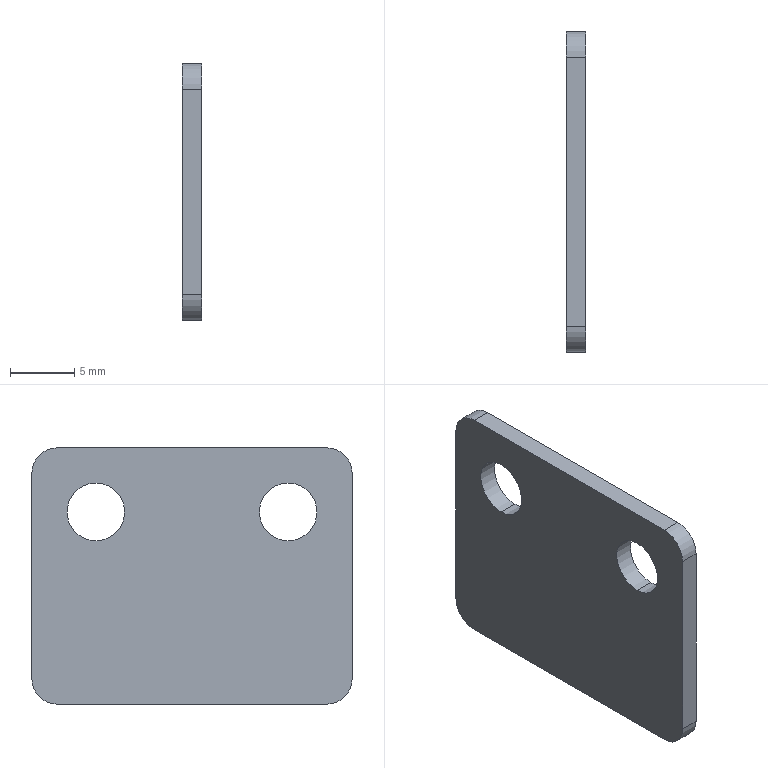Part | SolidWorks | features BaseBody 1 | 1 solid | 14 faces | box 1.5 x 25 x 20 mm | volume 697.137 mm3 | cylinder 8 | plane 6 | commonest cylinder face diameters 4 x4 4.5 x4
STEP:
#1=CARTESIAN_POINT('',(0.,12.5,-2.));
#2=VERTEX_POINT('',#1);
#3=CARTESIAN_POINT('',(0.,10.5,0.));
#4=VERTEX_POINT('',#3);
#5=CARTESIAN_POINT('',(0.,10.5,-2.));
#6=DIRECTION('',(1.,0.,0.));
#7=DIRECTION('',(0.,0.,-1.));
#8=AXIS2_PLACEMENT_3D('',#5,#6,#7);
#9=CIRCLE('',#8,2.);
#10=EDGE_CURVE('',#2,#4,#9,.T.);
#11=ORIENTED_EDGE('',*,*,#10,.F.);
#12=CARTESIAN_POINT('',(-1.5,12.5,-2.));
#13=VERTEX_POINT('',#12);
#14=CARTESIAN_POINT('',(0.,12.5,-2.));
#15=DIRECTION('',(1.,0.,0.));
#16=VECTOR('',#15,1000.);
#17=LINE('',#14,#16);
#18=EDGE_CURVE('',#13,#2,#17,.T.);
#19=ORIENTED_EDGE('',*,*,#18,.F.);
#20=CARTESIAN_POINT('',(-1.5,10.5,0.));
#21=VERTEX_POINT('',#20);
#22=CARTESIAN_POINT('',(-1.5,10.5,-2.));
#23=DIRECTION('',(-1.,0.,0.));
#24=DIRECTION('',(0.,0.,-1.));
#25=AXIS2_PLACEMENT_3D('',#22,#23,#24);
#26=CIRCLE('',#25,2.);
#27=EDGE_CURVE('',#21,#13,#26,.T.);
#28=ORIENTED_EDGE('',*,*,#27,.F.);
#29=CARTESIAN_POINT('',(0.,10.5,0.));
#30=DIRECTION('',(-1.,0.,0.));
#31=VECTOR('',#30,1000.);
#32=LINE('',#29,#31);
#33=EDGE_CURVE('',#4,#21,#32,.T.);
#34=ORIENTED_EDGE('',*,*,#33,.F.);
#35=EDGE_LOOP('',(#11,#19,#28,#34));
#36=FACE_OUTER_BOUND('',#35,.T.);
#37=CARTESIAN_POINT('',(0.,10.5,-2.));
#38=DIRECTION('',(-1.,0.,0.));
#39=DIRECTION('',(0.,0.,1.));
#40=AXIS2_PLACEMENT_3D('',#37,#38,#39);
#41=CYLINDRICAL_SURFACE('',#40,2.);
#42=ADVANCED_FACE('',(#36),#41,.T.);
#43=CARTESIAN_POINT('',(0.,-10.5,0.));
#44=VERTEX_POINT('',#43);
#45=CARTESIAN_POINT('',(0.,-12.5,-2.));
#46=VERTEX_POINT('',#45);
#47=CARTESIAN_POINT('',(0.,-10.5,-2.));
#48=DIRECTION('',(1.,0.,0.));
#49=DIRECTION('',(0.,0.,-1.));
#50=AXIS2_PLACEMENT_3D('',#47,#48,#49);
#51=CIRCLE('',#50,2.);
#52=EDGE_CURVE('',#44,#46,#51,.T.);
#53=ORIENTED_EDGE('',*,*,#52,.F.);
#54=CARTESIAN_POINT('',(-1.5,-10.5,0.));
#55=VERTEX_POINT('',#54);
#56=CARTESIAN_POINT('',(0.,-10.5,0.));
#57=DIRECTION('',(1.,0.,0.));
#58=VECTOR('',#57,1000.);
#59=LINE('',#56,#58);
#60=EDGE_CURVE('',#55,#44,#59,.T.);
#61=ORIENTED_EDGE('',*,*,#60,.F.);
#62=CARTESIAN_POINT('',(-1.5,-12.5,-2.));
#63=VERTEX_POINT('',#62);
#64=CARTESIAN_POINT('',(-1.5,-10.5,-2.));
#65=DIRECTION('',(-1.,0.,0.));
#66=DIRECTION('',(0.,0.,-1.));
#67=AXIS2_PLACEMENT_3D('',#64,#65,#66);
#68=CIRCLE('',#67,2.);
#69=EDGE_CURVE('',#63,#55,#68,.T.);
#70=ORIENTED_EDGE('',*,*,#69,.F.);
#71=CARTESIAN_POINT('',(-1.5,-12.5,-2.));
#72=DIRECTION('',(-1.,0.,0.));
#73=VECTOR('',#72,1000.);
#74=LINE('',#71,#73);
#75=EDGE_CURVE('',#46,#63,#74,.T.);
#76=ORIENTED_EDGE('',*,*,#75,.F.);
#77=EDGE_LOOP('',(#53,#61,#70,#76));
#78=FACE_OUTER_BOUND('',#77,.T.);
#79=CARTESIAN_POINT('',(0.,-10.5,-2.));
#80=DIRECTION('',(1.,0.,0.));
#81=DIRECTION('',(0.,0.,-1.));
#82=AXIS2_PLACEMENT_3D('',#79,#80,#81);
#83=CYLINDRICAL_SURFACE('',#82,2.);
#84=ADVANCED_FACE('',(#78),#83,.T.);
#85=CARTESIAN_POINT('',(-1.5,12.5,-18.));
#86=VERTEX_POINT('',#85);
#87=CARTESIAN_POINT('',(-1.5,10.5,-20.));
#88=VERTEX_POINT('',#87);
#89=CARTESIAN_POINT('',(-1.5,10.5,-18.));
#90=DIRECTION('',(-1.,0.,0.));
#91=DIRECTION('',(0.,0.,-1.));
#92=AXIS2_PLACEMENT_3D('',#89,#90,#91);
#93=CIRCLE('',#92,2.);
#94=EDGE_CURVE('',#86,#88,#93,.T.);
#95=ORIENTED_EDGE('',*,*,#94,.F.);
#96=CARTESIAN_POINT('',(0.,12.5,-18.));
#97=VERTEX_POINT('',#96);
#98=CARTESIAN_POINT('',(0.,12.5,-18.));
#99=DIRECTION('',(-1.,0.,0.));
#100=VECTOR('',#99,1000.);
#101=LINE('',#98,#100);
#102=EDGE_CURVE('',#97,#86,#101,.T.);
#103=ORIENTED_EDGE('',*,*,#102,.F.);
#104=CARTESIAN_POINT('',(0.,10.5,-20.));
#105=VERTEX_POINT('',#104);
#106=CARTESIAN_POINT('',(0.,10.5,-18.));
#107=DIRECTION('',(1.,0.,0.));
#108=DIRECTION('',(0.,0.,-1.));
#109=AXIS2_PLACEMENT_3D('',#106,#107,#108);
#110=CIRCLE('',#109,2.);
#111=EDGE_CURVE('',#105,#97,#110,.T.);
#112=ORIENTED_EDGE('',*,*,#111,.F.);
#113=CARTESIAN_POINT('',(-1.5,10.5,-20.));
#114=DIRECTION('',(1.,0.,0.));
#115=VECTOR('',#114,1000.);
#116=LINE('',#113,#115);
#117=EDGE_CURVE('',#88,#105,#116,.T.);
#118=ORIENTED_EDGE('',*,*,#117,.F.);
#119=EDGE_LOOP('',(#95,#103,#112,#118));
#120=FACE_OUTER_BOUND('',#119,.T.);
#121=CARTESIAN_POINT('',(-1.5,10.5,-18.));
#122=DIRECTION('',(1.,0.,0.));
#123=DIRECTION('',(0.,0.,-1.));
#124=AXIS2_PLACEMENT_3D('',#121,#122,#123);
#125=CYLINDRICAL_SURFACE('',#124,2.);
#126=ADVANCED_FACE('',(#120),#125,.T.);
#127=CARTESIAN_POINT('',(-1.5,-10.5,-20.));
#128=VERTEX_POINT('',#127);
#129=CARTESIAN_POINT('',(-1.5,-12.5,-18.));
#130=VERTEX_POINT('',#129);
#131=CARTESIAN_POINT('',(-1.5,-10.5,-18.));
#132=DIRECTION('',(-1.,0.,0.));
#133=DIRECTION('',(0.,0.,-1.));
#134=AXIS2_PLACEMENT_3D('',#131,#132,#133);
#135=CIRCLE('',#134,2.);
#136=EDGE_CURVE('',#128,#130,#135,.T.);
#137=ORIENTED_EDGE('',*,*,#136,.F.);
#138=CARTESIAN_POINT('',(0.,-10.5,-20.));
#139=VERTEX_POINT('',#138);
#140=CARTESIAN_POINT('',(-1.5,-10.5,-20.));
#141=DIRECTION('',(-1.,0.,0.));
#142=VECTOR('',#141,1000.);
#143=LINE('',#140,#142);
#144=EDGE_CURVE('',#139,#128,#143,.T.);
#145=ORIENTED_EDGE('',*,*,#144,.F.);
#146=CARTESIAN_POINT('',(0.,-12.5,-18.));
#147=VERTEX_POINT('',#146);
#148=CARTESIAN_POINT('',(0.,-10.5,-18.));
#149=DIRECTION('',(1.,0.,0.));
#150=DIRECTION('',(0.,0.,-1.));
#151=AXIS2_PLACEMENT_3D('',#148,#149,#150);
#152=CIRCLE('',#151,2.);
#153=EDGE_CURVE('',#147,#139,#152,.T.);
#154=ORIENTED_EDGE('',*,*,#153,.F.);
#155=CARTESIAN_POINT('',(0.,-12.5,-18.));
#156=DIRECTION('',(1.,0.,0.));
#157=VECTOR('',#156,1000.);
#158=LINE('',#155,#157);
#159=EDGE_CURVE('',#130,#147,#158,.T.);
#160=ORIENTED_EDGE('',*,*,#159,.F.);
#161=EDGE_LOOP('',(#137,#145,#154,#160));
#162=FACE_OUTER_BOUND('',#161,.T.);
#163=CARTESIAN_POINT('',(0.,-10.5,-18.));
#164=DIRECTION('',(-1.,0.,0.));
#165=DIRECTION('',(0.,0.,1.));
#166=AXIS2_PLACEMENT_3D('',#163,#164,#165);
#167=CYLINDRICAL_SURFACE('',#166,2.);
#168=ADVANCED_FACE('',(#162),#167,.T.);
#169=CARTESIAN_POINT('',(-1.5,-7.5,-2.75));
#170=VERTEX_POINT('',#169);
#171=CARTESIAN_POINT('',(0.,-7.5,-2.75));
#172=VERTEX_POINT('',#171);
#173=CARTESIAN_POINT('',(0.,-7.5,-2.75));
#174=DIRECTION('',(1.,0.,0.));
#175=VECTOR('',#174,1000.);
#176=LINE('',#173,#175);
#177=EDGE_CURVE('',#170,#172,#176,.T.);
#178=ORIENTED_EDGE('',*,*,#177,.F.);
#179=CARTESIAN_POINT('',(-1.5,-7.5,-7.25));
#180=VERTEX_POINT('',#179);
#181=CARTESIAN_POINT('',(-1.5,-7.5,-5.));
#182=DIRECTION('',(1.,0.,0.));
#183=DIRECTION('',(0.,0.,-1.));
#184=AXIS2_PLACEMENT_3D('',#181,#182,#183);
#185=CIRCLE('',#184,2.25);
#186=EDGE_CURVE('',#180,#170,#185,.T.);
#187=ORIENTED_EDGE('',*,*,#186,.F.);
#188=CARTESIAN_POINT('',(0.,-7.5,-7.25));
#189=VERTEX_POINT('',#188);
#190=CARTESIAN_POINT('',(0.,-7.5,-7.25));
#191=DIRECTION('',(1.,0.,0.));
#192=VECTOR('',#191,1000.);
#193=LINE('',#190,#192);
#194=EDGE_CURVE('',#180,#189,#193,.T.);
#195=ORIENTED_EDGE('',*,*,#194,.T.);
#196=CARTESIAN_POINT('',(0.,-7.5,-5.));
#197=DIRECTION('',(1.,0.,0.));
#198=DIRECTION('',(0.,0.,-1.));
#199=AXIS2_PLACEMENT_3D('',#196,#197,#198);
#200=CIRCLE('',#199,2.25);
#201=EDGE_CURVE('',#189,#172,#200,.T.);
#202=ORIENTED_EDGE('',*,*,#201,.T.);
#203=EDGE_LOOP('',(#178,#187,#195,#202));
#204=FACE_OUTER_BOUND('',#203,.T.);
#205=CARTESIAN_POINT('',(0.,-7.5,-5.));
#206=DIRECTION('',(1.,0.,0.));
#207=DIRECTION('',(0.,0.,-1.));
#208=AXIS2_PLACEMENT_3D('',#205,#206,#207);
#209=CYLINDRICAL_SURFACE('',#208,2.25);
#210=ADVANCED_FACE('',(#204),#209,.F.);
#211=CARTESIAN_POINT('',(-1.5,7.5,-2.75));
#212=VERTEX_POINT('',#211);
#213=CARTESIAN_POINT('',(0.,7.5,-2.75));
#214=VERTEX_POINT('',#213);
#215=CARTESIAN_POINT('',(0.,7.5,-2.75));
#216=DIRECTION('',(1.,0.,0.));
#217=VECTOR('',#216,1000.);
#218=LINE('',#215,#217);
#219=EDGE_CURVE('',#212,#214,#218,.T.);
#220=ORIENTED_EDGE('',*,*,#219,.F.);
#221=CARTESIAN_POINT('',(-1.5,7.5,-7.25));
#222=VERTEX_POINT('',#221);
#223=CARTESIAN_POINT('',(-1.5,7.5,-5.));
#224=DIRECTION('',(1.,0.,0.));
#225=DIRECTION('',(0.,0.,-1.));
#226=AXIS2_PLACEMENT_3D('',#223,#224,#225);
#227=CIRCLE('',#226,2.25);
#228=EDGE_CURVE('',#222,#212,#227,.T.);
#229=ORIENTED_EDGE('',*,*,#228,.F.);
#230=CARTESIAN_POINT('',(0.,7.5,-7.25));
#231=VERTEX_POINT('',#230);
#232=CARTESIAN_POINT('',(0.,7.5,-7.25));
#233=DIRECTION('',(1.,0.,0.));
#234=VECTOR('',#233,1000.);
#235=LINE('',#232,#234);
#236=EDGE_CURVE('',#222,#231,#235,.T.);
#237=ORIENTED_EDGE('',*,*,#236,.T.);
#238=CARTESIAN_POINT('',(0.,7.5,-5.));
#239=DIRECTION('',(1.,0.,0.));
#240=DIRECTION('',(0.,0.,-1.));
#241=AXIS2_PLACEMENT_3D('',#238,#239,#240);
#242=CIRCLE('',#241,2.25);
#243=EDGE_CURVE('',#231,#214,#242,.T.);
#244=ORIENTED_EDGE('',*,*,#243,.T.);
#245=EDGE_LOOP('',(#220,#229,#237,#244));
#246=FACE_OUTER_BOUND('',#245,.T.);
#247=CARTESIAN_POINT('',(0.,7.5,-5.));
#248=DIRECTION('',(1.,0.,0.));
#249=DIRECTION('',(0.,0.,-1.));
#250=AXIS2_PLACEMENT_3D('',#247,#248,#249);
#251=CYLINDRICAL_SURFACE('',#250,2.25);
#252=ADVANCED_FACE('',(#246),#251,.F.);
#253=CARTESIAN_POINT('',(-1.5,-12.5,-20.));
#254=DIRECTION('',(0.,0.,1.));
#255=VECTOR('',#254,1000.);
#256=LINE('',#253,#255);
#257=EDGE_CURVE('',#130,#63,#256,.T.);
#258=ORIENTED_EDGE('',*,*,#257,.F.);
#259=ORIENTED_EDGE('',*,*,#159,.T.);
#260=CARTESIAN_POINT('',(0.,-12.5,-20.));
#261=DIRECTION('',(0.,0.,1.));
#262=VECTOR('',#261,1000.);
#263=LINE('',#260,#262);
#264=EDGE_CURVE('',#147,#46,#263,.T.);
#265=ORIENTED_EDGE('',*,*,#264,.T.);
#266=ORIENTED_EDGE('',*,*,#75,.T.);
#267=EDGE_LOOP('',(#258,#259,#265,#266));
#268=FACE_OUTER_BOUND('',#267,.T.);
#269=CARTESIAN_POINT('',(0.,-12.5,0.));
#270=DIRECTION('',(0.,1.,0.));
#271=DIRECTION('',(1.,0.,0.));
#272=AXIS2_PLACEMENT_3D('',#269,#270,#271);
#273=PLANE('',#272);
#274=ADVANCED_FACE('',(#268),#273,.F.);
#275=CARTESIAN_POINT('',(0.,12.5,-20.));
#276=DIRECTION('',(0.,0.,1.));
#277=VECTOR('',#276,1000.);
#278=LINE('',#275,#277);
#279=EDGE_CURVE('',#97,#2,#278,.T.);
#280=ORIENTED_EDGE('',*,*,#279,.F.);
#281=ORIENTED_EDGE('',*,*,#102,.T.);
#282=CARTESIAN_POINT('',(-1.5,12.5,-20.));
#283=DIRECTION('',(0.,0.,1.));
#284=VECTOR('',#283,1000.);
#285=LINE('',#282,#284);
#286=EDGE_CURVE('',#86,#13,#285,.T.);
#287=ORIENTED_EDGE('',*,*,#286,.T.);
#288=ORIENTED_EDGE('',*,*,#18,.T.);
#289=EDGE_LOOP('',(#280,#281,#287,#288));
#290=FACE_OUTER_BOUND('',#289,.T.);
#291=CARTESIAN_POINT('',(0.,12.5,0.));
#292=DIRECTION('',(0.,1.,0.));
#293=DIRECTION('',(1.,0.,0.));
#294=AXIS2_PLACEMENT_3D('',#291,#292,#293);
#295=PLANE('',#294);
#296=ADVANCED_FACE('',(#290),#295,.T.);
#297=CARTESIAN_POINT('',(0.,12.5,-20.));
#298=DIRECTION('',(0.,-1.,0.));
#299=VECTOR('',#298,1000.);
#300=LINE('',#297,#299);
#301=EDGE_CURVE('',#105,#139,#300,.T.);
#302=ORIENTED_EDGE('',*,*,#301,.T.);
#303=ORIENTED_EDGE('',*,*,#144,.T.);
#304=CARTESIAN_POINT('',(-1.5,12.5,-20.));
#305=DIRECTION('',(0.,-1.,0.));
#306=VECTOR('',#305,1000.);
#307=LINE('',#304,#306);
#308=EDGE_CURVE('',#88,#128,#307,.T.);
#309=ORIENTED_EDGE('',*,*,#308,.F.);
#310=ORIENTED_EDGE('',*,*,#117,.T.);
#311=EDGE_LOOP('',(#302,#303,#309,#310));
#312=FACE_OUTER_BOUND('',#311,.T.);
#313=CARTESIAN_POINT('',(-1.5,12.5,-20.));
#314=DIRECTION('',(0.,0.,-1.));
#315=DIRECTION('',(0.,-1.,0.));
#316=AXIS2_PLACEMENT_3D('',#313,#314,#315);
#317=PLANE('',#316);
#318=ADVANCED_FACE('',(#312),#317,.T.);
#319=ORIENTED_EDGE('',*,*,#243,.F.);
#320=CARTESIAN_POINT('',(0.,7.5,-5.));
#321=DIRECTION('',(1.,0.,0.));
#322=DIRECTION('',(0.,0.,-1.));
#323=AXIS2_PLACEMENT_3D('',#320,#321,#322);
#324=CIRCLE('',#323,2.25);
#325=EDGE_CURVE('',#214,#231,#324,.T.);
#326=ORIENTED_EDGE('',*,*,#325,.F.);
#327=EDGE_LOOP('',(#319,#326));
#328=FACE_BOUND('',#327,.T.);
#329=ORIENTED_EDGE('',*,*,#201,.F.);
#330=CARTESIAN_POINT('',(0.,-7.5,-5.));
#331=DIRECTION('',(1.,0.,0.));
#332=DIRECTION('',(0.,0.,-1.));
#333=AXIS2_PLACEMENT_3D('',#330,#331,#332);
#334=CIRCLE('',#333,2.25);
#335=EDGE_CURVE('',#172,#189,#334,.T.);
#336=ORIENTED_EDGE('',*,*,#335,.F.);
#337=EDGE_LOOP('',(#329,#336));
#338=FACE_BOUND('',#337,.T.);
#339=ORIENTED_EDGE('',*,*,#264,.F.);
#340=ORIENTED_EDGE('',*,*,#153,.T.);
#341=ORIENTED_EDGE('',*,*,#301,.F.);
#342=ORIENTED_EDGE('',*,*,#111,.T.);
#343=ORIENTED_EDGE('',*,*,#279,.T.);
#344=ORIENTED_EDGE('',*,*,#10,.T.);
#345=CARTESIAN_POINT('',(0.,12.5,0.));
#346=DIRECTION('',(0.,-1.,0.));
#347=VECTOR('',#346,1000.);
#348=LINE('',#345,#347);
#349=EDGE_CURVE('',#4,#44,#348,.T.);
#350=ORIENTED_EDGE('',*,*,#349,.T.);
#351=ORIENTED_EDGE('',*,*,#52,.T.);
#352=EDGE_LOOP('',(#339,#340,#341,#342,#343,#344,#350,#351));
#353=FACE_OUTER_BOUND('',#352,.T.);
#354=CARTESIAN_POINT('',(0.,12.5,-20.));
#355=DIRECTION('',(1.,0.,0.));
#356=DIRECTION('',(0.,1.,0.));
#357=AXIS2_PLACEMENT_3D('',#354,#355,#356);
#358=PLANE('',#357);
#359=ADVANCED_FACE('',(#328,#338,#353),#358,.T.);
#360=CARTESIAN_POINT('',(-1.5,12.5,0.));
#361=DIRECTION('',(0.,-1.,0.));
#362=VECTOR('',#361,1000.);
#363=LINE('',#360,#362);
#364=EDGE_CURVE('',#21,#55,#363,.T.);
#365=ORIENTED_EDGE('',*,*,#364,.T.);
#366=ORIENTED_EDGE('',*,*,#60,.T.);
#367=ORIENTED_EDGE('',*,*,#349,.F.);
#368=ORIENTED_EDGE('',*,*,#33,.T.);
#369=EDGE_LOOP('',(#365,#366,#367,#368));
#370=FACE_OUTER_BOUND('',#369,.T.);
#371=CARTESIAN_POINT('',(0.,12.5,0.));
#372=DIRECTION('',(0.,0.,1.));
#373=DIRECTION('',(1.,0.,0.));
#374=AXIS2_PLACEMENT_3D('',#371,#372,#373);
#375=PLANE('',#374);
#376=ADVANCED_FACE('',(#370),#375,.T.);
#377=ORIENTED_EDGE('',*,*,#228,.T.);
#378=CARTESIAN_POINT('',(-1.5,7.5,-5.));
#379=DIRECTION('',(1.,0.,0.));
#380=DIRECTION('',(0.,0.,-1.));
#381=AXIS2_PLACEMENT_3D('',#378,#379,#380);
#382=CIRCLE('',#381,2.25);
#383=EDGE_CURVE('',#212,#222,#382,.T.);
#384=ORIENTED_EDGE('',*,*,#383,.T.);
#385=EDGE_LOOP('',(#377,#384));
#386=FACE_BOUND('',#385,.T.);
#387=ORIENTED_EDGE('',*,*,#186,.T.);
#388=CARTESIAN_POINT('',(-1.5,-7.5,-5.));
#389=DIRECTION('',(1.,0.,0.));
#390=DIRECTION('',(0.,0.,-1.));
#391=AXIS2_PLACEMENT_3D('',#388,#389,#390);
#392=CIRCLE('',#391,2.25);
#393=EDGE_CURVE('',#170,#180,#392,.T.);
#394=ORIENTED_EDGE('',*,*,#393,.T.);
#395=EDGE_LOOP('',(#387,#394));
#396=FACE_BOUND('',#395,.T.);
#397=ORIENTED_EDGE('',*,*,#308,.T.);
#398=ORIENTED_EDGE('',*,*,#136,.T.);
#399=ORIENTED_EDGE('',*,*,#257,.T.);
#400=ORIENTED_EDGE('',*,*,#69,.T.);
#401=ORIENTED_EDGE('',*,*,#364,.F.);
#402=ORIENTED_EDGE('',*,*,#27,.T.);
#403=ORIENTED_EDGE('',*,*,#286,.F.);
#404=ORIENTED_EDGE('',*,*,#94,.T.);
#405=EDGE_LOOP('',(#397,#398,#399,#400,#401,#402,#403,#404));
#406=FACE_OUTER_BOUND('',#405,.T.);
#407=CARTESIAN_POINT('',(-1.5,12.5,-20.));
#408=DIRECTION('',(1.,0.,0.));
#409=DIRECTION('',(0.,1.,0.));
#410=AXIS2_PLACEMENT_3D('',#407,#408,#409);
#411=PLANE('',#410);
#412=ADVANCED_FACE('',(#386,#396,#406),#411,.F.);
#413=ORIENTED_EDGE('',*,*,#383,.F.);
#414=ORIENTED_EDGE('',*,*,#219,.T.);
#415=ORIENTED_EDGE('',*,*,#325,.T.);
#416=ORIENTED_EDGE('',*,*,#236,.F.);
#417=EDGE_LOOP('',(#413,#414,#415,#416));
#418=FACE_OUTER_BOUND('',#417,.T.);
#419=CARTESIAN_POINT('',(0.,7.5,-5.));
#420=DIRECTION('',(1.,0.,0.));
#421=DIRECTION('',(0.,0.,-1.));
#422=AXIS2_PLACEMENT_3D('',#419,#420,#421);
#423=CYLINDRICAL_SURFACE('',#422,2.25);
#424=ADVANCED_FACE('',(#418),#423,.F.);
#425=ORIENTED_EDGE('',*,*,#393,.F.);
#426=ORIENTED_EDGE('',*,*,#177,.T.);
#427=ORIENTED_EDGE('',*,*,#335,.T.);
#428=ORIENTED_EDGE('',*,*,#194,.F.);
#429=EDGE_LOOP('',(#425,#426,#427,#428));
#430=FACE_OUTER_BOUND('',#429,.T.);
#431=CARTESIAN_POINT('',(0.,-7.5,-5.));
#432=DIRECTION('',(1.,0.,0.));
#433=DIRECTION('',(0.,0.,-1.));
#434=AXIS2_PLACEMENT_3D('',#431,#432,#433);
#435=CYLINDRICAL_SURFACE('',#434,2.25);
#436=ADVANCED_FACE('',(#430),#435,.F.);
#437=CLOSED_SHELL('',(#42,#84,#126,#168,#210,#252,#274,#296,#318,#359,#376,#412,#424,#436));
#438=MANIFOLD_SOLID_BREP('',#437);
#439=CARTESIAN_POINT('',(0.,0.,0.));
#440=DIRECTION('',(0.,0.,1.));
#441=DIRECTION('',(1.,0.,0.));
#442=AXIS2_PLACEMENT_3D('',#439,#440,#441);
#443=(LENGTH_UNIT()NAMED_UNIT(*)SI_UNIT(.MILLI.,.METRE.));
#444=UNCERTAINTY_MEASURE_WITH_UNIT(LENGTH_MEASURE(0.00001),#443,'','');
#445=(NAMED_UNIT(*)PLANE_ANGLE_UNIT()SI_UNIT($,.RADIAN.));
#446=(NAMED_UNIT(*)SI_UNIT($,.STERADIAN.)SOLID_ANGLE_UNIT());
#447=(GEOMETRIC_REPRESENTATION_CONTEXT(3)GLOBAL_UNCERTAINTY_ASSIGNED_CONTEXT((#444))GLOBAL_UNIT_ASSIGNED_CONTEXT((#443,#445,#446))REPRESENTATION_CONTEXT('',''));
#448=ADVANCED_BREP_SHAPE_REPRESENTATION('',(#438,#442),#447);